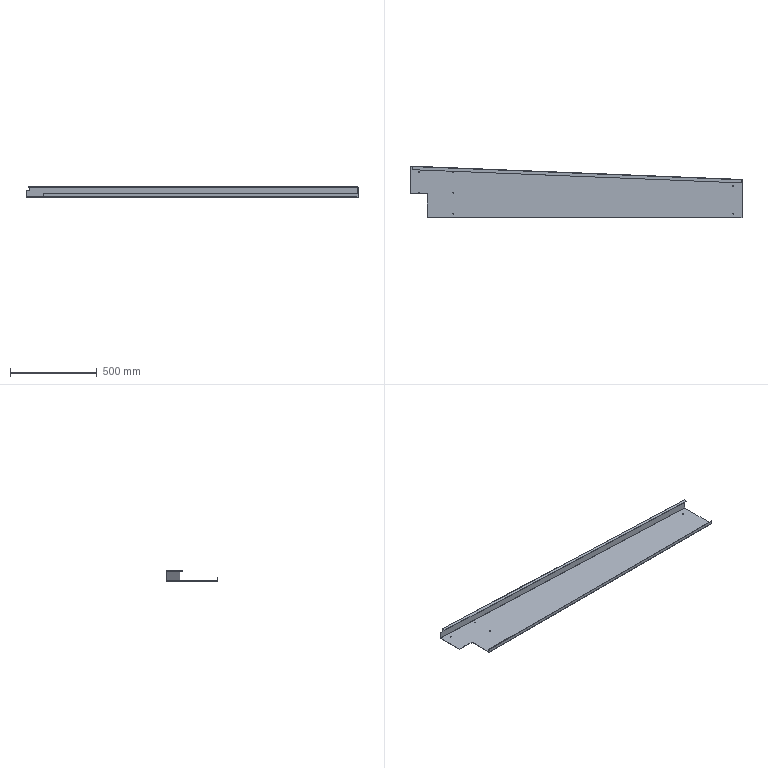Part | STEP file | TS-S17 | 1 solid | 49 faces | box 1915 x 298.7 x 60 mm | volume 1317864 mm3 | plane 28 | cylinder 20 | spline 1 | commonest cylinder face diameters 5.4 x14 0.4 x3 4.4 x3